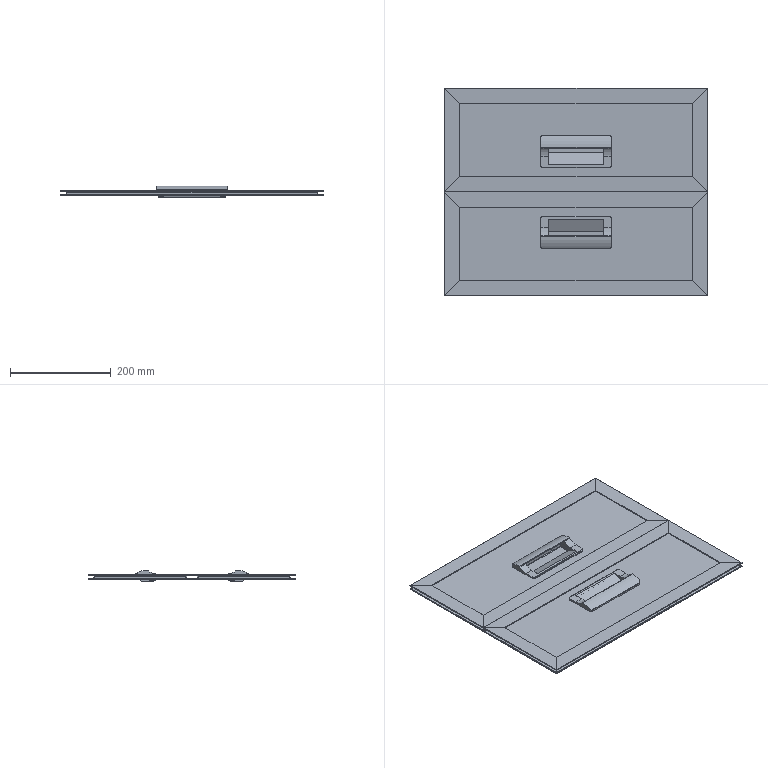Part | SolidWorks | 12 solids | 318 faces | box 520 x 410 x 23.592 mm | volume 1199217 mm3 | plane 206 | cylinder 88 | spline 8 | cone 8 | torus 8 | commonest cylinder face diameters 2 x44 4 x8 8 x8 10 x8 12 x8 52 x6